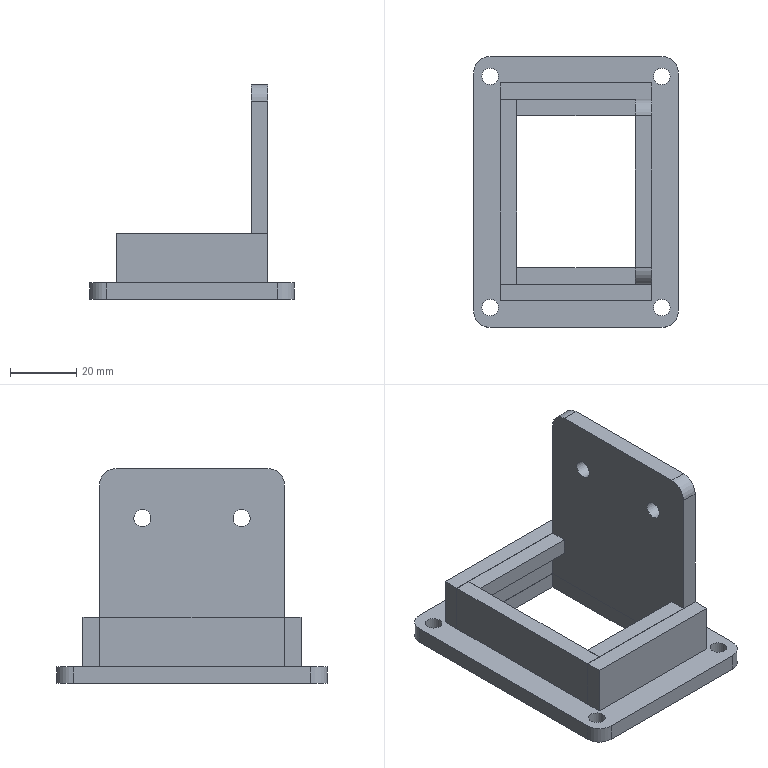Part | NX | features BREP 7 | 7 solids | 58 faces | box 62 x 82 x 65 mm | volume 44274 mm3 | plane 46 | cylinder 12 | commonest cylinder face diameters 10 x6 5 x4 5.2 x2
STEP:
#1=CARTESIAN_POINT('',(23.,-28.,5.));
#2=VERTEX_POINT('',#1);
#3=CARTESIAN_POINT('',(-23.,-28.,5.));
#4=VERTEX_POINT('',#3);
#5=CARTESIAN_POINT('',(-23.,-28.,5.));
#6=DIRECTION('',(-1.,0.,0.));
#7=VECTOR('',#6,1000.);
#8=LINE('',#5,#7);
#9=EDGE_CURVE('',#2,#4,#8,.T.);
#10=ORIENTED_EDGE('',*,*,#9,.T.);
#11=CARTESIAN_POINT('',(-23.,-28.,20.));
#12=VERTEX_POINT('',#11);
#13=CARTESIAN_POINT('',(-23.,-28.,20.));
#14=DIRECTION('',(0.,0.,-1.));
#15=VECTOR('',#14,1000.);
#16=LINE('',#13,#15);
#17=EDGE_CURVE('',#12,#4,#16,.T.);
#18=ORIENTED_EDGE('',*,*,#17,.F.);
#19=CARTESIAN_POINT('',(23.,-28.,20.));
#20=VERTEX_POINT('',#19);
#21=CARTESIAN_POINT('',(-23.,-28.,20.));
#22=DIRECTION('',(-1.,0.,0.));
#23=VECTOR('',#22,1000.);
#24=LINE('',#21,#23);
#25=EDGE_CURVE('',#20,#12,#24,.T.);
#26=ORIENTED_EDGE('',*,*,#25,.F.);
#27=CARTESIAN_POINT('',(23.,-28.,20.));
#28=DIRECTION('',(0.,0.,-1.));
#29=VECTOR('',#28,1000.);
#30=LINE('',#27,#29);
#31=EDGE_CURVE('',#20,#2,#30,.T.);
#32=ORIENTED_EDGE('',*,*,#31,.T.);
#33=EDGE_LOOP('',(#10,#18,#26,#32));
#34=FACE_BOUND('',#33,.T.);
#35=CARTESIAN_POINT('',(-23.,-28.,20.));
#36=DIRECTION('',(0.,-1.,0.));
#37=DIRECTION('',(0.,0.,-1.));
#38=AXIS2_PLACEMENT_3D('',#35,#36,#37);
#39=PLANE('',#38);
#40=ADVANCED_FACE('',(#34),#39,.F.);
#41=CARTESIAN_POINT('',(-23.,-33.,5.));
#42=VERTEX_POINT('',#41);
#43=CARTESIAN_POINT('',(-23.,-28.,5.));
#44=DIRECTION('',(0.,-1.,0.));
#45=VECTOR('',#44,1000.);
#46=LINE('',#43,#45);
#47=EDGE_CURVE('',#4,#42,#46,.T.);
#48=ORIENTED_EDGE('',*,*,#47,.T.);
#49=CARTESIAN_POINT('',(-23.,-33.,20.));
#50=VERTEX_POINT('',#49);
#51=CARTESIAN_POINT('',(-23.,-33.,20.));
#52=DIRECTION('',(0.,0.,-1.));
#53=VECTOR('',#52,1000.);
#54=LINE('',#51,#53);
#55=EDGE_CURVE('',#50,#42,#54,.T.);
#56=ORIENTED_EDGE('',*,*,#55,.F.);
#57=CARTESIAN_POINT('',(-23.,-28.,20.));
#58=DIRECTION('',(0.,-1.,0.));
#59=VECTOR('',#58,1000.);
#60=LINE('',#57,#59);
#61=EDGE_CURVE('',#12,#50,#60,.T.);
#62=ORIENTED_EDGE('',*,*,#61,.F.);
#63=ORIENTED_EDGE('',*,*,#17,.T.);
#64=EDGE_LOOP('',(#48,#56,#62,#63));
#65=FACE_BOUND('',#64,.T.);
#66=CARTESIAN_POINT('',(-23.,-28.,20.));
#67=DIRECTION('',(1.,0.,0.));
#68=DIRECTION('',(0.,0.,-1.));
#69=AXIS2_PLACEMENT_3D('',#66,#67,#68);
#70=PLANE('',#69);
#71=ADVANCED_FACE('',(#65),#70,.F.);
#72=CARTESIAN_POINT('',(23.,-33.,5.));
#73=VERTEX_POINT('',#72);
#74=CARTESIAN_POINT('',(-23.,-33.,5.));
#75=DIRECTION('',(1.,0.,0.));
#76=VECTOR('',#75,1000.);
#77=LINE('',#74,#76);
#78=EDGE_CURVE('',#42,#73,#77,.T.);
#79=ORIENTED_EDGE('',*,*,#78,.T.);
#80=CARTESIAN_POINT('',(23.,-33.,20.));
#81=VERTEX_POINT('',#80);
#82=CARTESIAN_POINT('',(23.,-33.,20.));
#83=DIRECTION('',(0.,0.,-1.));
#84=VECTOR('',#83,1000.);
#85=LINE('',#82,#84);
#86=EDGE_CURVE('',#81,#73,#85,.T.);
#87=ORIENTED_EDGE('',*,*,#86,.F.);
#88=CARTESIAN_POINT('',(-23.,-33.,20.));
#89=DIRECTION('',(1.,0.,0.));
#90=VECTOR('',#89,1000.);
#91=LINE('',#88,#90);
#92=EDGE_CURVE('',#50,#81,#91,.T.);
#93=ORIENTED_EDGE('',*,*,#92,.F.);
#94=ORIENTED_EDGE('',*,*,#55,.T.);
#95=EDGE_LOOP('',(#79,#87,#93,#94));
#96=FACE_BOUND('',#95,.T.);
#97=CARTESIAN_POINT('',(-23.,-33.,20.));
#98=DIRECTION('',(0.,1.,0.));
#99=DIRECTION('',(0.,0.,1.));
#100=AXIS2_PLACEMENT_3D('',#97,#98,#99);
#101=PLANE('',#100);
#102=ADVANCED_FACE('',(#96),#101,.F.);
#103=CARTESIAN_POINT('',(23.,-28.,5.));
#104=DIRECTION('',(0.,1.,0.));
#105=VECTOR('',#104,1000.);
#106=LINE('',#103,#105);
#107=EDGE_CURVE('',#73,#2,#106,.T.);
#108=ORIENTED_EDGE('',*,*,#107,.T.);
#109=ORIENTED_EDGE('',*,*,#31,.F.);
#110=CARTESIAN_POINT('',(23.,-28.,20.));
#111=DIRECTION('',(0.,1.,0.));
#112=VECTOR('',#111,1000.);
#113=LINE('',#110,#112);
#114=EDGE_CURVE('',#81,#20,#113,.T.);
#115=ORIENTED_EDGE('',*,*,#114,.F.);
#116=ORIENTED_EDGE('',*,*,#86,.T.);
#117=EDGE_LOOP('',(#108,#109,#115,#116));
#118=FACE_BOUND('',#117,.T.);
#119=CARTESIAN_POINT('',(23.,-28.,20.));
#120=DIRECTION('',(-1.,0.,0.));
#121=DIRECTION('',(0.,0.,1.));
#122=AXIS2_PLACEMENT_3D('',#119,#120,#121);
#123=PLANE('',#122);
#124=ADVANCED_FACE('',(#118),#123,.F.);
#125=ORIENTED_EDGE('',*,*,#25,.T.);
#126=ORIENTED_EDGE('',*,*,#61,.T.);
#127=ORIENTED_EDGE('',*,*,#92,.T.);
#128=ORIENTED_EDGE('',*,*,#114,.T.);
#129=EDGE_LOOP('',(#125,#126,#127,#128));
#130=FACE_BOUND('',#129,.T.);
#131=CARTESIAN_POINT('',(0.,0.,20.));
#132=DIRECTION('',(0.,0.,-1.));
#133=DIRECTION('',(-1.,0.,0.));
#134=AXIS2_PLACEMENT_3D('',#131,#132,#133);
#135=PLANE('',#134);
#136=ADVANCED_FACE('',(#130),#135,.F.);
#137=ORIENTED_EDGE('',*,*,#9,.F.);
#138=ORIENTED_EDGE('',*,*,#107,.F.);
#139=ORIENTED_EDGE('',*,*,#78,.F.);
#140=ORIENTED_EDGE('',*,*,#47,.F.);
#141=EDGE_LOOP('',(#137,#138,#139,#140));
#142=FACE_BOUND('',#141,.T.);
#143=CARTESIAN_POINT('',(0.,0.,5.));
#144=DIRECTION('',(0.,0.,-1.));
#145=DIRECTION('',(-1.,0.,0.));
#146=AXIS2_PLACEMENT_3D('',#143,#144,#145);
#147=PLANE('',#146);
#148=ADVANCED_FACE('',(#142),#147,.T.);
#149=CLOSED_SHELL('',(#40,#71,#102,#124,#136,#148));
#150=MANIFOLD_SOLID_BREP('',#149);
#151=CARTESIAN_POINT('',(-18.,-28.,20.));
#152=VERTEX_POINT('',#151);
#153=CARTESIAN_POINT('',(18.,-28.,20.));
#154=VERTEX_POINT('',#153);
#155=CARTESIAN_POINT('',(-18.,-28.,20.));
#156=DIRECTION('',(1.,0.,0.));
#157=VECTOR('',#156,1000.);
#158=LINE('',#155,#157);
#159=EDGE_CURVE('',#152,#154,#158,.T.);
#160=ORIENTED_EDGE('',*,*,#159,.F.);
#161=CARTESIAN_POINT('',(-18.,-28.,15.));
#162=VERTEX_POINT('',#161);
#163=CARTESIAN_POINT('',(-18.,-28.,15.));
#164=DIRECTION('',(0.,0.,1.));
#165=VECTOR('',#164,1000.);
#166=LINE('',#163,#165);
#167=EDGE_CURVE('',#162,#152,#166,.T.);
#168=ORIENTED_EDGE('',*,*,#167,.F.);
#169=CARTESIAN_POINT('',(18.,-28.,15.));
#170=VERTEX_POINT('',#169);
#171=CARTESIAN_POINT('',(-18.,-28.,15.));
#172=DIRECTION('',(1.,0.,0.));
#173=VECTOR('',#172,1000.);
#174=LINE('',#171,#173);
#175=EDGE_CURVE('',#162,#170,#174,.T.);
#176=ORIENTED_EDGE('',*,*,#175,.T.);
#177=CARTESIAN_POINT('',(18.,-28.,15.));
#178=DIRECTION('',(0.,0.,1.));
#179=VECTOR('',#178,1000.);
#180=LINE('',#177,#179);
#181=EDGE_CURVE('',#170,#154,#180,.T.);
#182=ORIENTED_EDGE('',*,*,#181,.T.);
#183=EDGE_LOOP('',(#160,#168,#176,#182));
#184=FACE_BOUND('',#183,.T.);
#185=CARTESIAN_POINT('',(-18.,-28.,15.));
#186=DIRECTION('',(0.,-1.,0.));
#187=DIRECTION('',(0.,0.,-1.));
#188=AXIS2_PLACEMENT_3D('',#185,#186,#187);
#189=PLANE('',#188);
#190=ADVANCED_FACE('',(#184),#189,.T.);
#191=CARTESIAN_POINT('',(-18.,-23.,20.));
#192=VERTEX_POINT('',#191);
#193=CARTESIAN_POINT('',(-18.,-28.,20.));
#194=DIRECTION('',(0.,-1.,0.));
#195=VECTOR('',#194,1000.);
#196=LINE('',#193,#195);
#197=EDGE_CURVE('',#192,#152,#196,.T.);
#198=ORIENTED_EDGE('',*,*,#197,.F.);
#199=CARTESIAN_POINT('',(-18.,-23.,15.));
#200=VERTEX_POINT('',#199);
#201=CARTESIAN_POINT('',(-18.,-23.,15.));
#202=DIRECTION('',(0.,0.,1.));
#203=VECTOR('',#202,1000.);
#204=LINE('',#201,#203);
#205=EDGE_CURVE('',#200,#192,#204,.T.);
#206=ORIENTED_EDGE('',*,*,#205,.F.);
#207=CARTESIAN_POINT('',(-18.,-28.,15.));
#208=DIRECTION('',(0.,-1.,0.));
#209=VECTOR('',#208,1000.);
#210=LINE('',#207,#209);
#211=EDGE_CURVE('',#200,#162,#210,.T.);
#212=ORIENTED_EDGE('',*,*,#211,.T.);
#213=ORIENTED_EDGE('',*,*,#167,.T.);
#214=EDGE_LOOP('',(#198,#206,#212,#213));
#215=FACE_BOUND('',#214,.T.);
#216=CARTESIAN_POINT('',(-18.,-28.,15.));
#217=DIRECTION('',(-1.,0.,0.));
#218=DIRECTION('',(0.,0.,1.));
#219=AXIS2_PLACEMENT_3D('',#216,#217,#218);
#220=PLANE('',#219);
#221=ADVANCED_FACE('',(#215),#220,.T.);
#222=CARTESIAN_POINT('',(18.,-23.,20.));
#223=VERTEX_POINT('',#222);
#224=CARTESIAN_POINT('',(-18.,-23.,20.));
#225=DIRECTION('',(-1.,0.,0.));
#226=VECTOR('',#225,1000.);
#227=LINE('',#224,#226);
#228=EDGE_CURVE('',#223,#192,#227,.T.);
#229=ORIENTED_EDGE('',*,*,#228,.F.);
#230=CARTESIAN_POINT('',(18.,-23.,15.));
#231=VERTEX_POINT('',#230);
#232=CARTESIAN_POINT('',(18.,-23.,15.));
#233=DIRECTION('',(0.,0.,1.));
#234=VECTOR('',#233,1000.);
#235=LINE('',#232,#234);
#236=EDGE_CURVE('',#231,#223,#235,.T.);
#237=ORIENTED_EDGE('',*,*,#236,.F.);
#238=CARTESIAN_POINT('',(-18.,-23.,15.));
#239=DIRECTION('',(-1.,0.,0.));
#240=VECTOR('',#239,1000.);
#241=LINE('',#238,#240);
#242=EDGE_CURVE('',#231,#200,#241,.T.);
#243=ORIENTED_EDGE('',*,*,#242,.T.);
#244=ORIENTED_EDGE('',*,*,#205,.T.);
#245=EDGE_LOOP('',(#229,#237,#243,#244));
#246=FACE_BOUND('',#245,.T.);
#247=CARTESIAN_POINT('',(-18.,-23.,15.));
#248=DIRECTION('',(0.,1.,0.));
#249=DIRECTION('',(0.,0.,1.));
#250=AXIS2_PLACEMENT_3D('',#247,#248,#249);
#251=PLANE('',#250);
#252=ADVANCED_FACE('',(#246),#251,.T.);
#253=CARTESIAN_POINT('',(18.,-28.,20.));
#254=DIRECTION('',(0.,1.,0.));
#255=VECTOR('',#254,1000.);
#256=LINE('',#253,#255);
#257=EDGE_CURVE('',#154,#223,#256,.T.);
#258=ORIENTED_EDGE('',*,*,#257,.F.);
#259=ORIENTED_EDGE('',*,*,#181,.F.);
#260=CARTESIAN_POINT('',(18.,-28.,15.));
#261=DIRECTION('',(0.,1.,0.));
#262=VECTOR('',#261,1000.);
#263=LINE('',#260,#262);
#264=EDGE_CURVE('',#170,#231,#263,.T.);
#265=ORIENTED_EDGE('',*,*,#264,.T.);
#266=ORIENTED_EDGE('',*,*,#236,.T.);
#267=EDGE_LOOP('',(#258,#259,#265,#266));
#268=FACE_BOUND('',#267,.T.);
#269=CARTESIAN_POINT('',(18.,-28.,15.));
#270=DIRECTION('',(1.,0.,0.));
#271=DIRECTION('',(0.,1.,0.));
#272=AXIS2_PLACEMENT_3D('',#269,#270,#271);
#273=PLANE('',#272);
#274=ADVANCED_FACE('',(#268),#273,.T.);
#275=ORIENTED_EDGE('',*,*,#175,.F.);
#276=ORIENTED_EDGE('',*,*,#211,.F.);
#277=ORIENTED_EDGE('',*,*,#242,.F.);
#278=ORIENTED_EDGE('',*,*,#264,.F.);
#279=EDGE_LOOP('',(#275,#276,#277,#278));
#280=FACE_BOUND('',#279,.T.);
#281=CARTESIAN_POINT('',(0.,0.,15.));
#282=DIRECTION('',(0.,0.,1.));
#283=DIRECTION('',(1.,0.,0.));
#284=AXIS2_PLACEMENT_3D('',#281,#282,#283);
#285=PLANE('',#284);
#286=ADVANCED_FACE('',(#280),#285,.F.);
#287=ORIENTED_EDGE('',*,*,#159,.T.);
#288=ORIENTED_EDGE('',*,*,#257,.T.);
#289=ORIENTED_EDGE('',*,*,#228,.T.);
#290=ORIENTED_EDGE('',*,*,#197,.T.);
#291=EDGE_LOOP('',(#287,#288,#289,#290));
#292=FACE_BOUND('',#291,.T.);
#293=CARTESIAN_POINT('',(0.,0.,20.));
#294=DIRECTION('',(0.,0.,1.));
#295=DIRECTION('',(1.,0.,0.));
#296=AXIS2_PLACEMENT_3D('',#293,#294,#295);
#297=PLANE('',#296);
#298=ADVANCED_FACE('',(#292),#297,.T.);
#299=CLOSED_SHELL('',(#190,#221,#252,#274,#286,#298));
#300=MANIFOLD_SOLID_BREP('',#299);
#301=CARTESIAN_POINT('',(23.,15.,47.4));
#302=VERTEX_POINT('',#301);
#303=CARTESIAN_POINT('',(23.,15.,50.));
#304=DIRECTION('',(1.,0.,0.));
#305=DIRECTION('',(0.,0.,-1.));
#306=AXIS2_PLACEMENT_3D('',#303,#304,#305);
#307=CIRCLE('',#306,2.6);
#308=EDGE_CURVE('',#302,#302,#307,.T.);
#309=ORIENTED_EDGE('',*,*,#308,.T.);
#310=EDGE_LOOP('',(#309));
#311=FACE_BOUND('',#310,.T.);
#312=CARTESIAN_POINT('',(18.,15.,47.4));
#313=VERTEX_POINT('',#312);
#314=CARTESIAN_POINT('',(18.,15.,50.));
#315=DIRECTION('',(1.,0.,0.));
#316=DIRECTION('',(0.,0.,-1.));
#317=AXIS2_PLACEMENT_3D('',#314,#315,#316);
#318=CIRCLE('',#317,2.6);
#319=EDGE_CURVE('',#313,#313,#318,.T.);
#320=ORIENTED_EDGE('',*,*,#319,.F.);
#321=EDGE_LOOP('',(#320));
#322=FACE_BOUND('',#321,.T.);
#323=CARTESIAN_POINT('',(23.,15.,50.));
#324=DIRECTION('',(1.,0.,0.));
#325=DIRECTION('',(0.,0.,-1.));
#326=AXIS2_PLACEMENT_3D('',#323,#324,#325);
#327=CYLINDRICAL_SURFACE('',#326,2.6);
#328=ADVANCED_FACE('',(#311,#322),#327,.F.);
#329=CARTESIAN_POINT('',(23.,-15.,47.4));
#330=VERTEX_POINT('',#329);
#331=CARTESIAN_POINT('',(23.,-15.,50.));
#332=DIRECTION('',(1.,0.,0.));
#333=DIRECTION('',(0.,0.,-1.));
#334=AXIS2_PLACEMENT_3D('',#331,#332,#333);
#335=CIRCLE('',#334,2.6);
#336=EDGE_CURVE('',#330,#330,#335,.T.);
#337=ORIENTED_EDGE('',*,*,#336,.T.);
#338=EDGE_LOOP('',(#337));
#339=FACE_BOUND('',#338,.T.);
#340=CARTESIAN_POINT('',(18.,-15.,47.4));
#341=VERTEX_POINT('',#340);
#342=CARTESIAN_POINT('',(18.,-15.,50.));
#343=DIRECTION('',(1.,0.,0.));
#344=DIRECTION('',(0.,0.,-1.));
#345=AXIS2_PLACEMENT_3D('',#342,#343,#344);
#346=CIRCLE('',#345,2.6);
#347=EDGE_CURVE('',#341,#341,#346,.T.);
#348=ORIENTED_EDGE('',*,*,#347,.F.);
#349=EDGE_LOOP('',(#348));
#350=FACE_BOUND('',#349,.T.);
#351=CARTESIAN_POINT('',(23.,-15.,50.));
#352=DIRECTION('',(1.,0.,0.));
#353=DIRECTION('',(0.,0.,-1.));
#354=AXIS2_PLACEMENT_3D('',#351,#352,#353);
#355=CYLINDRICAL_SURFACE('',#354,2.6);
#356=ADVANCED_FACE('',(#339,#350),#355,.F.);
#357=ORIENTED_EDGE('',*,*,#308,.F.);
#358=EDGE_LOOP('',(#357));
#359=FACE_BOUND('',#358,.T.);
#360=ORIENTED_EDGE('',*,*,#336,.F.);
#361=EDGE_LOOP('',(#360));
#362=FACE_BOUND('',#361,.T.);
#363=CARTESIAN_POINT('',(23.,28.,60.));
#364=VERTEX_POINT('',#363);
#365=CARTESIAN_POINT('',(23.,28.,5.));
#366=VERTEX_POINT('',#365);
#367=CARTESIAN_POINT('',(23.,28.,65.));
#368=DIRECTION('',(0.,0.,-1.));
#369=VECTOR('',#368,1000.);
#370=LINE('',#367,#369);
#371=EDGE_CURVE('',#364,#366,#370,.T.);
#372=ORIENTED_EDGE('',*,*,#371,.F.);
#373=CARTESIAN_POINT('',(23.,23.,65.));
#374=VERTEX_POINT('',#373);
#375=CARTESIAN_POINT('',(23.,23.,60.));
#376=DIRECTION('',(1.,0.,0.));
#377=DIRECTION('',(0.,0.,1.));
#378=AXIS2_PLACEMENT_3D('',#375,#376,#377);
#379=CIRCLE('',#378,5.);
#380=EDGE_CURVE('',#364,#374,#379,.T.);
#381=ORIENTED_EDGE('',*,*,#380,.T.);
#382=CARTESIAN_POINT('',(23.,-23.,65.));
#383=VERTEX_POINT('',#382);
#384=CARTESIAN_POINT('',(23.,-28.,65.));
#385=DIRECTION('',(0.,1.,0.));
#386=VECTOR('',#385,1000.);
#387=LINE('',#384,#386);
#388=EDGE_CURVE('',#383,#374,#387,.T.);
#389=ORIENTED_EDGE('',*,*,#388,.F.);
#390=CARTESIAN_POINT('',(23.,-28.,60.));
#391=VERTEX_POINT('',#390);
#392=CARTESIAN_POINT('',(23.,-23.,60.));
#393=DIRECTION('',(1.,0.,0.));
#394=DIRECTION('',(0.,0.,1.));
#395=AXIS2_PLACEMENT_3D('',#392,#393,#394);
#396=CIRCLE('',#395,5.);
#397=EDGE_CURVE('',#383,#391,#396,.T.);
#398=ORIENTED_EDGE('',*,*,#397,.T.);
#399=CARTESIAN_POINT('',(23.,-28.,5.));
#400=VERTEX_POINT('',#399);
#401=CARTESIAN_POINT('',(23.,-28.,65.));
#402=DIRECTION('',(0.,0.,-1.));
#403=VECTOR('',#402,1000.);
#404=LINE('',#401,#403);
#405=EDGE_CURVE('',#391,#400,#404,.T.);
#406=ORIENTED_EDGE('',*,*,#405,.T.);
#407=CARTESIAN_POINT('',(23.,28.,5.));
#408=DIRECTION('',(0.,1.,0.));
#409=VECTOR('',#408,1000.);
#410=LINE('',#407,#409);
#411=EDGE_CURVE('',#400,#366,#410,.T.);
#412=ORIENTED_EDGE('',*,*,#411,.T.);
#413=EDGE_LOOP('',(#372,#381,#389,#398,#406,#412));
#414=FACE_BOUND('',#413,.T.);
#415=CARTESIAN_POINT('',(23.,-28.,65.));
#416=DIRECTION('',(-1.,0.,0.));
#417=DIRECTION('',(0.,0.,1.));
#418=AXIS2_PLACEMENT_3D('',#415,#416,#417);
#419=PLANE('',#418);
#420=ADVANCED_FACE('',(#359,#362,#414),#419,.F.);
#421=CARTESIAN_POINT('',(18.,28.,60.));
#422=VERTEX_POINT('',#421);
#423=CARTESIAN_POINT('',(18.,28.,5.));
#424=VERTEX_POINT('',#423);
#425=CARTESIAN_POINT('',(18.,28.,65.));
#426=DIRECTION('',(0.,0.,-1.));
#427=VECTOR('',#426,1000.);
#428=LINE('',#425,#427);
#429=EDGE_CURVE('',#422,#424,#428,.T.);
#430=ORIENTED_EDGE('',*,*,#429,.F.);
#431=CARTESIAN_POINT('',(23.,28.,60.));
#432=DIRECTION('',(1.,0.,0.));
#433=VECTOR('',#432,1000.);
#434=LINE('',#431,#433);
#435=EDGE_CURVE('',#422,#364,#434,.T.);
#436=ORIENTED_EDGE('',*,*,#435,.T.);
#437=ORIENTED_EDGE('',*,*,#371,.T.);
#438=CARTESIAN_POINT('',(18.,28.,5.));
#439=DIRECTION('',(-1.,0.,0.));
#440=VECTOR('',#439,1000.);
#441=LINE('',#438,#440);
#442=EDGE_CURVE('',#366,#424,#441,.T.);
#443=ORIENTED_EDGE('',*,*,#442,.T.);
#444=EDGE_LOOP('',(#430,#436,#437,#443));
#445=FACE_BOUND('',#444,.T.);
#446=CARTESIAN_POINT('',(23.,28.,65.));
#447=DIRECTION('',(0.,-1.,0.));
#448=DIRECTION('',(0.,0.,-1.));
#449=AXIS2_PLACEMENT_3D('',#446,#447,#448);
#450=PLANE('',#449);
#451=ADVANCED_FACE('',(#445),#450,.F.);
#452=ORIENTED_EDGE('',*,*,#319,.T.);
#453=EDGE_LOOP('',(#452));
#454=FACE_BOUND('',#453,.T.);
#455=ORIENTED_EDGE('',*,*,#347,.T.);
#456=EDGE_LOOP('',(#455));
#457=FACE_BOUND('',#456,.T.);
#458=CARTESIAN_POINT('',(18.,23.,65.));
#459=VERTEX_POINT('',#458);
#460=CARTESIAN_POINT('',(18.,-23.,65.));
#461=VERTEX_POINT('',#460);
#462=CARTESIAN_POINT('',(18.,-28.,65.));
#463=DIRECTION('',(0.,-1.,0.));
#464=VECTOR('',#463,1000.);
#465=LINE('',#462,#464);
#466=EDGE_CURVE('',#459,#461,#465,.T.);
#467=ORIENTED_EDGE('',*,*,#466,.F.);
#468=CARTESIAN_POINT('',(18.,23.,60.));
#469=DIRECTION('',(-1.,0.,0.));
#470=DIRECTION('',(0.,0.,-1.));
#471=AXIS2_PLACEMENT_3D('',#468,#469,#470);
#472=CIRCLE('',#471,5.);
#473=EDGE_CURVE('',#459,#422,#472,.T.);
#474=ORIENTED_EDGE('',*,*,#473,.T.);
#475=ORIENTED_EDGE('',*,*,#429,.T.);
#476=CARTESIAN_POINT('',(18.,-28.,5.));
#477=VERTEX_POINT('',#476);
#478=CARTESIAN_POINT('',(18.,28.,5.));
#479=DIRECTION('',(0.,-1.,0.));
#480=VECTOR('',#479,1000.);
#481=LINE('',#478,#480);
#482=EDGE_CURVE('',#424,#477,#481,.T.);
#483=ORIENTED_EDGE('',*,*,#482,.T.);
#484=CARTESIAN_POINT('',(18.,-28.,60.));
#485=VERTEX_POINT('',#484);
#486=CARTESIAN_POINT('',(18.,-28.,65.));
#487=DIRECTION('',(0.,0.,-1.));
#488=VECTOR('',#487,1000.);
#489=LINE('',#486,#488);
#490=EDGE_CURVE('',#485,#477,#489,.T.);
#491=ORIENTED_EDGE('',*,*,#490,.F.);
#492=CARTESIAN_POINT('',(18.,-23.,60.));
#493=DIRECTION('',(-1.,0.,0.));
#494=DIRECTION('',(0.,0.,-1.));
#495=AXIS2_PLACEMENT_3D('',#492,#493,#494);
#496=CIRCLE('',#495,5.);
#497=EDGE_CURVE('',#485,#461,#496,.T.);
#498=ORIENTED_EDGE('',*,*,#497,.T.);
#499=EDGE_LOOP('',(#467,#474,#475,#483,#491,#498));
#500=FACE_BOUND('',#499,.T.);
#501=CARTESIAN_POINT('',(18.,-28.,65.));
#502=DIRECTION('',(1.,0.,0.));
#503=DIRECTION('',(0.,0.,-1.));
#504=AXIS2_PLACEMENT_3D('',#501,#502,#503);
#505=PLANE('',#504);
#506=ADVANCED_FACE('',(#454,#457,#500),#505,.F.);
#507=ORIENTED_EDGE('',*,*,#405,.F.);
#508=CARTESIAN_POINT('',(18.,-28.,60.));
#509=DIRECTION('',(-1.,0.,0.));
#510=VECTOR('',#509,1000.);
#511=LINE('',#508,#510);
#512=EDGE_CURVE('',#391,#485,#511,.T.);
#513=ORIENTED_EDGE('',*,*,#512,.T.);
#514=ORIENTED_EDGE('',*,*,#490,.T.);
#515=CARTESIAN_POINT('',(18.,-28.,5.));
#516=DIRECTION('',(1.,0.,0.));
#517=VECTOR('',#516,1000.);
#518=LINE('',#515,#517);
#519=EDGE_CURVE('',#477,#400,#518,.T.);
#520=ORIENTED_EDGE('',*,*,#519,.T.);
#521=EDGE_LOOP('',(#507,#513,#514,#520));
#522=FACE_BOUND('',#521,.T.);
#523=CARTESIAN_POINT('',(23.,-28.,65.));
#524=DIRECTION('',(0.,1.,0.));
#525=DIRECTION('',(0.,0.,1.));
#526=AXIS2_PLACEMENT_3D('',#523,#524,#525);
#527=PLANE('',#526);
#528=ADVANCED_FACE('',(#522),#527,.F.);
#529=ORIENTED_EDGE('',*,*,#388,.T.);
#530=CARTESIAN_POINT('',(18.,23.,65.));
#531=DIRECTION('',(-1.,0.,0.));
#532=VECTOR('',#531,1000.);
#533=LINE('',#530,#532);
#534=EDGE_CURVE('',#374,#459,#533,.T.);
#535=ORIENTED_EDGE('',*,*,#534,.T.);
#536=ORIENTED_EDGE('',*,*,#466,.T.);
#537=CARTESIAN_POINT('',(23.,-23.,65.));
#538=DIRECTION('',(1.,0.,0.));
#539=VECTOR('',#538,1000.);
#540=LINE('',#537,#539);
#541=EDGE_CURVE('',#461,#383,#540,.T.);
#542=ORIENTED_EDGE('',*,*,#541,.T.);
#543=EDGE_LOOP('',(#529,#535,#536,#542));
#544=FACE_BOUND('',#543,.T.);
#545=CARTESIAN_POINT('',(0.,0.,65.));
#546=DIRECTION('',(0.,0.,1.));
#547=DIRECTION('',(1.,0.,0.));
#548=AXIS2_PLACEMENT_3D('',#545,#546,#547);
#549=PLANE('',#548);
#550=ADVANCED_FACE('',(#544),#549,.T.);
#551=ORIENTED_EDGE('',*,*,#380,.F.);
#552=ORIENTED_EDGE('',*,*,#435,.F.);
#553=ORIENTED_EDGE('',*,*,#473,.F.);
#554=ORIENTED_EDGE('',*,*,#534,.F.);
#555=EDGE_LOOP('',(#551,#552,#553,#554));
#556=FACE_BOUND('',#555,.T.);
#557=CARTESIAN_POINT('',(0.,23.,60.));
#558=DIRECTION('',(1.,0.,0.));
#559=DIRECTION('',(0.,0.,-1.));
#560=AXIS2_PLACEMENT_3D('',#557,#558,#559);
#561=CYLINDRICAL_SURFACE('',#560,5.);
#562=ADVANCED_FACE('',(#556),#561,.T.);
#563=ORIENTED_EDGE('',*,*,#497,.F.);
#564=ORIENTED_EDGE('',*,*,#512,.F.);
#565=ORIENTED_EDGE('',*,*,#397,.F.);
#566=ORIENTED_EDGE('',*,*,#541,.F.);
#567=EDGE_LOOP('',(#563,#564,#565,#566));
#568=FACE_BOUND('',#567,.T.);
#569=CARTESIAN_POINT('',(0.,-23.,60.));
#570=DIRECTION('',(-1.,0.,0.));
#571=DIRECTION('',(0.,0.,1.));
#572=AXIS2_PLACEMENT_3D('',#569,#570,#571);
#573=CYLINDRICAL_SURFACE('',#572,5.);
#574=ADVANCED_FACE('',(#568),#573,.T.);
#575=ORIENTED_EDGE('',*,*,#442,.F.);
#576=ORIENTED_EDGE('',*,*,#411,.F.);
#577=ORIENTED_EDGE('',*,*,#519,.F.);
#578=ORIENTED_EDGE('',*,*,#482,.F.);
#579=EDGE_LOOP('',(#575,#576,#577,#578));
#580=FACE_BOUND('',#579,.T.);
#581=CARTESIAN_POINT('',(0.,0.,5.));
#582=DIRECTION('',(0.,0.,-1.));
#583=DIRECTION('',(-1.,0.,0.));
#584=AXIS2_PLACEMENT_3D('',#581,#582,#583);
#585=PLANE('',#584);
#586=ADVANCED_FACE('',(#580),#585,.T.);
#587=CLOSED_SHELL('',(#328,#356,#420,#451,#506,#528,#550,#562,#574,#586));
#588=MANIFOLD_SOLID_BREP('',#587);
#589=CARTESIAN_POINT('',(-18.,-28.,5.));
#590=VERTEX_POINT('',#589);
#591=CARTESIAN_POINT('',(-18.,28.,5.));
#592=VERTEX_POINT('',#591);
#593=CARTESIAN_POINT('',(-18.,28.,5.));
#594=DIRECTION('',(0.,1.,0.));
#595=VECTOR('',#594,1000.);
#596=LINE('',#593,#595);
#597=EDGE_CURVE('',#590,#592,#596,.T.);
#598=ORIENTED_EDGE('',*,*,#597,.T.);
#599=CARTESIAN_POINT('',(-18.,28.,20.));
#600=VERTEX_POINT('',#599);
#601=CARTESIAN_POINT('',(-18.,28.,20.));
#602=DIRECTION('',(0.,0.,-1.));
#603=VECTOR('',#602,1000.);
#604=LINE('',#601,#603);
#605=EDGE_CURVE('',#600,#592,#604,.T.);
#606=ORIENTED_EDGE('',*,*,#605,.F.);
#607=CARTESIAN_POINT('',(-18.,-28.,20.));
#608=VERTEX_POINT('',#607);
#609=CARTESIAN_POINT('',(-18.,28.,20.));
#610=DIRECTION('',(0.,1.,0.));
#611=VECTOR('',#610,1000.);
#612=LINE('',#609,#611);
#613=EDGE_CURVE('',#608,#600,#612,.T.);
#614=ORIENTED_EDGE('',*,*,#613,.F.);
#615=CARTESIAN_POINT('',(-18.,-28.,20.));
#616=DIRECTION('',(0.,0.,-1.));
#617=VECTOR('',#616,1000.);
#618=LINE('',#615,#617);
#619=EDGE_CURVE('',#608,#590,#618,.T.);
#620=ORIENTED_EDGE('',*,*,#619,.T.);
#621=EDGE_LOOP('',(#598,#606,#614,#620));
#622=FACE_BOUND('',#621,.T.);
#623=CARTESIAN_POINT('',(-18.,28.,20.));
#624=DIRECTION('',(-1.,0.,0.));
#625=DIRECTION('',(0.,0.,1.));
#626=AXIS2_PLACEMENT_3D('',#623,#624,#625);
#627=PLANE('',#626);
#628=ADVANCED_FACE('',(#622),#627,.F.);
#629=CARTESIAN_POINT('',(-23.,28.,5.));
#630=VERTEX_POINT('',#629);
#631=CARTESIAN_POINT('',(-18.,28.,5.));
#632=DIRECTION('',(-1.,0.,0.));
#633=VECTOR('',#632,1000.);
#634=LINE('',#631,#633);
#635=EDGE_CURVE('',#592,#630,#634,.T.);
#636=ORIENTED_EDGE('',*,*,#635,.T.);
#637=CARTESIAN_POINT('',(-23.,28.,20.));
#638=VERTEX_POINT('',#637);
#639=CARTESIAN_POINT('',(-23.,28.,20.));
#640=DIRECTION('',(0.,0.,-1.));
#641=VECTOR('',#640,1000.);
#642=LINE('',#639,#641);
#643=EDGE_CURVE('',#638,#630,#642,.T.);
#644=ORIENTED_EDGE('',*,*,#643,.F.);
#645=CARTESIAN_POINT('',(-18.,28.,20.));
#646=DIRECTION('',(-1.,0.,0.));
#647=VECTOR('',#646,1000.);
#648=LINE('',#645,#647);
#649=EDGE_CURVE('',#600,#638,#648,.T.);
#650=ORIENTED_EDGE('',*,*,#649,.F.);
#651=ORIENTED_EDGE('',*,*,#605,.T.);
#652=EDGE_LOOP('',(#636,#644,#650,#651));
#653=FACE_BOUND('',#652,.T.);
#654=CARTESIAN_POINT('',(-18.,28.,20.));
#655=DIRECTION('',(0.,-1.,0.));
#656=DIRECTION('',(0.,0.,-1.));
#657=AXIS2_PLACEMENT_3D('',#654,#655,#656);
#658=PLANE('',#657);
#659=ADVANCED_FACE('',(#653),#658,.F.);
#660=CARTESIAN_POINT('',(-23.,-28.,5.));
#661=VERTEX_POINT('',#660);
#662=CARTESIAN_POINT('',(-23.,28.,5.));
#663=DIRECTION('',(0.,-1.,0.));
#664=VECTOR('',#663,1000.);
#665=LINE('',#662,#664);
#666=EDGE_CURVE('',#630,#661,#665,.T.);
#667=ORIENTED_EDGE('',*,*,#666,.T.);
#668=CARTESIAN_POINT('',(-23.,-28.,20.));
#669=VERTEX_POINT('',#668);
#670=CARTESIAN_POINT('',(-23.,-28.,20.));
#671=DIRECTION('',(0.,0.,-1.));
#672=VECTOR('',#671,1000.);
#673=LINE('',#670,#672);
#674=EDGE_CURVE('',#669,#661,#673,.T.);
#675=ORIENTED_EDGE('',*,*,#674,.F.);
#676=CARTESIAN_POINT('',(-23.,28.,20.));
#677=DIRECTION('',(0.,-1.,0.));
#678=VECTOR('',#677,1000.);
#679=LINE('',#676,#678);
#680=EDGE_CURVE('',#638,#669,#679,.T.);
#681=ORIENTED_EDGE('',*,*,#680,.F.);
#682=ORIENTED_EDGE('',*,*,#643,.T.);
#683=EDGE_LOOP('',(#667,#675,#681,#682));
#684=FACE_BOUND('',#683,.T.);
#685=CARTESIAN_POINT('',(-23.,28.,20.));
#686=DIRECTION('',(1.,0.,0.));
#687=DIRECTION('',(0.,1.,0.));
#688=AXIS2_PLACEMENT_3D('',#685,#686,#687);
#689=PLANE('',#688);
#690=ADVANCED_FACE('',(#684),#689,.F.);
#691=CARTESIAN_POINT('',(-18.,-28.,5.));
#692=DIRECTION('',(1.,0.,0.));
#693=VECTOR('',#692,1000.);
#694=LINE('',#691,#693);
#695=EDGE_CURVE('',#661,#590,#694,.T.);
#696=ORIENTED_EDGE('',*,*,#695,.T.);
#697=ORIENTED_EDGE('',*,*,#619,.F.);
#698=CARTESIAN_POINT('',(-18.,-28.,20.));
#699=DIRECTION('',(1.,0.,0.));
#700=VECTOR('',#699,1000.);
#701=LINE('',#698,#700);
#702=EDGE_CURVE('',#669,#608,#701,.T.);
#703=ORIENTED_EDGE('',*,*,#702,.F.);
#704=ORIENTED_EDGE('',*,*,#674,.T.);
#705=EDGE_LOOP('',(#696,#697,#703,#704));
#706=FACE_BOUND('',#705,.T.);
#707=CARTESIAN_POINT('',(-18.,-28.,20.));
#708=DIRECTION('',(0.,1.,0.));
#709=DIRECTION('',(0.,0.,1.));
#710=AXIS2_PLACEMENT_3D('',#707,#708,#709);
#711=PLANE('',#710);
#712=ADVANCED_FACE('',(#706),#711,.F.);
#713=ORIENTED_EDGE('',*,*,#613,.T.);
#714=ORIENTED_EDGE('',*,*,#649,.T.);
#715=ORIENTED_EDGE('',*,*,#680,.T.);
#716=ORIENTED_EDGE('',*,*,#702,.T.);
#717=EDGE_LOOP('',(#713,#714,#715,#716));
#718=FACE_BOUND('',#717,.T.);
#719=CARTESIAN_POINT('',(0.,0.,20.));
#720=DIRECTION('',(0.,0.,-1.));
#721=DIRECTION('',(-1.,0.,0.));
#722=AXIS2_PLACEMENT_3D('',#719,#720,#721);
#723=PLANE('',#722);
#724=ADVANCED_FACE('',(#718),#723,.F.);
#725=ORIENTED_EDGE('',*,*,#597,.F.);
#726=ORIENTED_EDGE('',*,*,#695,.F.);
#727=ORIENTED_EDGE('',*,*,#666,.F.);
#728=ORIENTED_EDGE('',*,*,#635,.F.);
#729=EDGE_LOOP('',(#725,#726,#727,#728));
#730=FACE_BOUND('',#729,.T.);
#731=CARTESIAN_POINT('',(0.,0.,5.));
#732=DIRECTION('',(0.,0.,-1.));
#733=DIRECTION('',(-1.,0.,0.));
#734=AXIS2_PLACEMENT_3D('',#731,#732,#733);
#735=PLANE('',#734);
#736=ADVANCED_FACE('',(#730),#735,.T.);
#737=CLOSED_SHELL('',(#628,#659,#690,#712,#724,#736));
#738=MANIFOLD_SOLID_BREP('',#737);
#739=CARTESIAN_POINT('',(23.5,35.,0.));
#740=VERTEX_POINT('',#739);
#741=CARTESIAN_POINT('',(26.,35.,0.));
#742=DIRECTION('',(0.,0.,-1.));
#743=DIRECTION('',(-1.,0.,0.));
#744=AXIS2_PLACEMENT_3D('',#741,#742,#743);
#745=CIRCLE('',#744,2.5);
#746=EDGE_CURVE('',#740,#740,#745,.T.);
#747=ORIENTED_EDGE('',*,*,#746,.T.);
#748=EDGE_LOOP('',(#747));
#749=FACE_BOUND('',#748,.T.);
#750=CARTESIAN_POINT('',(28.5,35.,5.));
#751=VERTEX_POINT('',#750);
#752=CARTESIAN_POINT('',(26.,35.,5.));
#753=DIRECTION('',(0.,0.,-1.));
#754=DIRECTION('',(1.,0.,0.));
#755=AXIS2_PLACEMENT_3D('',#752,#753,#754);
#756=CIRCLE('',#755,2.5);
#757=EDGE_CURVE('',#751,#751,#756,.T.);
#758=ORIENTED_EDGE('',*,*,#757,.F.);
#759=EDGE_LOOP('',(#758));
#760=FACE_BOUND('',#759,.T.);
#761=CARTESIAN_POINT('',(26.,35.,0.));
#762=DIRECTION('',(0.,0.,-1.));
#763=DIRECTION('',(-1.,0.,0.));
#764=AXIS2_PLACEMENT_3D('',#761,#762,#763);
#765=CYLINDRICAL_SURFACE('',#764,2.5);
#766=ADVANCED_FACE('',(#749,#760),#765,.F.);
#767=CARTESIAN_POINT('',(-28.5,35.,0.));
#768=VERTEX_POINT('',#767);
#769=CARTESIAN_POINT('',(-26.,35.,0.));
#770=DIRECTION('',(0.,0.,-1.));
#771=DIRECTION('',(-1.,0.,0.));
#772=AXIS2_PLACEMENT_3D('',#769,#770,#771);
#773=CIRCLE('',#772,2.5);
#774=EDGE_CURVE('',#768,#768,#773,.T.);
#775=ORIENTED_EDGE('',*,*,#774,.T.);
#776=EDGE_LOOP('',(#775));
#777=FACE_BOUND('',#776,.T.);
#778=CARTESIAN_POINT('',(-23.5,35.,5.));
#779=VERTEX_POINT('',#778);
#780=CARTESIAN_POINT('',(-26.,35.,5.));
#781=DIRECTION('',(0.,0.,-1.));
#782=DIRECTION('',(1.,0.,0.));
#783=AXIS2_PLACEMENT_3D('',#780,#781,#782);
#784=CIRCLE('',#783,2.5);
#785=EDGE_CURVE('',#779,#779,#784,.T.);
#786=ORIENTED_EDGE('',*,*,#785,.F.);
#787=EDGE_LOOP('',(#786));
#788=FACE_BOUND('',#787,.T.);
#789=CARTESIAN_POINT('',(-26.,35.,0.));
#790=DIRECTION('',(0.,0.,-1.));
#791=DIRECTION('',(-1.,0.,0.));
#792=AXIS2_PLACEMENT_3D('',#789,#790,#791);
#793=CYLINDRICAL_SURFACE('',#792,2.5);
#794=ADVANCED_FACE('',(#777,#788),#793,.F.);
#795=CARTESIAN_POINT('',(-28.5,-35.,0.));
#796=VERTEX_POINT('',#795);
#797=CARTESIAN_POINT('',(-26.,-35.,0.));
#798=DIRECTION('',(0.,0.,-1.));
#799=DIRECTION('',(-1.,0.,0.));
#800=AXIS2_PLACEMENT_3D('',#797,#798,#799);
#801=CIRCLE('',#800,2.5);
#802=EDGE_CURVE('',#796,#796,#801,.T.);
#803=ORIENTED_EDGE('',*,*,#802,.T.);
#804=EDGE_LOOP('',(#803));
#805=FACE_BOUND('',#804,.T.);
#806=CARTESIAN_POINT('',(-23.5,-35.,5.));
#807=VERTEX_POINT('',#806);
#808=CARTESIAN_POINT('',(-26.,-35.,5.));
#809=DIRECTION('',(0.,0.,-1.));
#810=DIRECTION('',(1.,0.,0.));
#811=AXIS2_PLACEMENT_3D('',#808,#809,#810);
#812=CIRCLE('',#811,2.5);
#813=EDGE_CURVE('',#807,#807,#812,.T.);
#814=ORIENTED_EDGE('',*,*,#813,.F.);
#815=EDGE_LOOP('',(#814));
#816=FACE_BOUND('',#815,.T.);
#817=CARTESIAN_POINT('',(-26.,-35.,0.));
#818=DIRECTION('',(0.,0.,-1.));
#819=DIRECTION('',(-1.,0.,0.));
#820=AXIS2_PLACEMENT_3D('',#817,#818,#819);
#821=CYLINDRICAL_SURFACE('',#820,2.5);
#822=ADVANCED_FACE('',(#805,#816),#821,.F.);
#823=CARTESIAN_POINT('',(23.5,-35.,0.));
#824=VERTEX_POINT('',#823);
#825=CARTESIAN_POINT('',(26.,-35.,0.));
#826=DIRECTION('',(0.,0.,-1.));
#827=DIRECTION('',(-1.,0.,0.));
#828=AXIS2_PLACEMENT_3D('',#825,#826,#827);
#829=CIRCLE('',#828,2.5);
#830=EDGE_CURVE('',#824,#824,#829,.T.);
#831=ORIENTED_EDGE('',*,*,#830,.T.);
#832=EDGE_LOOP('',(#831));
#833=FACE_BOUND('',#832,.T.);
#834=CARTESIAN_POINT('',(28.5,-35.,5.));
#835=VERTEX_POINT('',#834);
#836=CARTESIAN_POINT('',(26.,-35.,5.));
#837=DIRECTION('',(0.,0.,-1.));
#838=DIRECTION('',(1.,0.,0.));
#839=AXIS2_PLACEMENT_3D('',#836,#837,#838);
#840=CIRCLE('',#839,2.5);
#841=EDGE_CURVE('',#835,#835,#840,.T.);
#842=ORIENTED_EDGE('',*,*,#841,.F.);
#843=EDGE_LOOP('',(#842));
#844=FACE_BOUND('',#843,.T.);
#845=CARTESIAN_POINT('',(26.,-35.,0.));
#846=DIRECTION('',(0.,0.,-1.));
#847=DIRECTION('',(-1.,0.,0.));
#848=AXIS2_PLACEMENT_3D('',#845,#846,#847);
#849=CYLINDRICAL_SURFACE('',#848,2.5);
#850=ADVANCED_FACE('',(#833,#844),#849,.F.);
#851=ORIENTED_EDGE('',*,*,#813,.T.);
#852=EDGE_LOOP('',(#851));
#853=FACE_BOUND('',#852,.T.);
#854=ORIENTED_EDGE('',*,*,#841,.T.);
#855=EDGE_LOOP('',(#854));
#856=FACE_BOUND('',#855,.T.);
#857=CARTESIAN_POINT('',(-31.,36.,5.));
#858=VERTEX_POINT('',#857);
#859=CARTESIAN_POINT('',(-31.,-36.,5.));
#860=VERTEX_POINT('',#859);
#861=CARTESIAN_POINT('',(-31.,-41.,5.));
#862=DIRECTION('',(0.,-1.,0.));
#863=VECTOR('',#862,1000.);
#864=LINE('',#861,#863);
#865=EDGE_CURVE('',#858,#860,#864,.T.);
#866=ORIENTED_EDGE('',*,*,#865,.T.);
#867=CARTESIAN_POINT('',(-26.,-41.,5.));
#868=VERTEX_POINT('',#867);
#869=CARTESIAN_POINT('',(-26.,-36.,5.));
#870=DIRECTION('',(0.,0.,1.));
#871=DIRECTION('',(1.,0.,0.));
#872=AXIS2_PLACEMENT_3D('',#869,#870,#871);
#873=CIRCLE('',#872,5.);
#874=EDGE_CURVE('',#860,#868,#873,.T.);
#875=ORIENTED_EDGE('',*,*,#874,.T.);
#876=CARTESIAN_POINT('',(26.,-41.,5.));
#877=VERTEX_POINT('',#876);
#878=CARTESIAN_POINT('',(-31.,-41.,5.));
#879=DIRECTION('',(1.,0.,0.));
#880=VECTOR('',#879,1000.);
#881=LINE('',#878,#880);
#882=EDGE_CURVE('',#868,#877,#881,.T.);
#883=ORIENTED_EDGE('',*,*,#882,.T.);
#884=CARTESIAN_POINT('',(31.,-36.,5.));
#885=VERTEX_POINT('',#884);
#886=CARTESIAN_POINT('',(26.,-36.,5.));
#887=DIRECTION('',(0.,0.,1.));
#888=DIRECTION('',(1.,0.,0.));
#889=AXIS2_PLACEMENT_3D('',#886,#887,#888);
#890=CIRCLE('',#889,5.);
#891=EDGE_CURVE('',#877,#885,#890,.T.);
#892=ORIENTED_EDGE('',*,*,#891,.T.);
#893=CARTESIAN_POINT('',(31.,36.,5.));
#894=VERTEX_POINT('',#893);
#895=CARTESIAN_POINT('',(31.,-41.,5.));
#896=DIRECTION('',(0.,1.,0.));
#897=VECTOR('',#896,1000.);
#898=LINE('',#895,#897);
#899=EDGE_CURVE('',#885,#894,#898,.T.);
#900=ORIENTED_EDGE('',*,*,#899,.T.);
#901=CARTESIAN_POINT('',(26.,41.,5.));
#902=VERTEX_POINT('',#901);
#903=CARTESIAN_POINT('',(26.,36.,5.));
#904=DIRECTION('',(0.,0.,1.));
#905=DIRECTION('',(1.,0.,0.));
#906=AXIS2_PLACEMENT_3D('',#903,#904,#905);
#907=CIRCLE('',#906,5.);
#908=EDGE_CURVE('',#894,#902,#907,.T.);
#909=ORIENTED_EDGE('',*,*,#908,.T.);
#910=CARTESIAN_POINT('',(-26.,41.,5.));
#911=VERTEX_POINT('',#910);
#912=CARTESIAN_POINT('',(-31.,41.,5.));
#913=DIRECTION('',(-1.,0.,0.));
#914=VECTOR('',#913,1000.);
#915=LINE('',#912,#914);
#916=EDGE_CURVE('',#902,#911,#915,.T.);
#917=ORIENTED_EDGE('',*,*,#916,.T.);
#918=CARTESIAN_POINT('',(-26.,36.,5.));
#919=DIRECTION('',(0.,0.,1.));
#920=DIRECTION('',(1.,0.,0.));
#921=AXIS2_PLACEMENT_3D('',#918,#919,#920);
#922=CIRCLE('',#921,5.);
#923=EDGE_CURVE('',#911,#858,#922,.T.);
#924=ORIENTED_EDGE('',*,*,#923,.T.);
#925=EDGE_LOOP('',(#866,#875,#883,#892,#900,#909,#917,#924));
#926=FACE_BOUND('',#925,.T.);
#927=CARTESIAN_POINT('',(-18.,28.,5.));
#928=VERTEX_POINT('',#927);
#929=CARTESIAN_POINT('',(-18.,-28.,5.));
#930=VERTEX_POINT('',#929);
#931=CARTESIAN_POINT('',(-18.,-28.,5.));
#932=DIRECTION('',(0.,-1.,0.));
#933=VECTOR('',#932,1000.);
#934=LINE('',#931,#933);
#935=EDGE_CURVE('',#928,#930,#934,.T.);
#936=ORIENTED_EDGE('',*,*,#935,.F.);
#937=CARTESIAN_POINT('',(18.,28.,5.));
#938=VERTEX_POINT('',#937);
#939=CARTESIAN_POINT('',(-18.,28.,5.));
#940=DIRECTION('',(-1.,0.,0.));
#941=VECTOR('',#940,1000.);
#942=LINE('',#939,#941);
#943=EDGE_CURVE('',#938,#928,#942,.T.);
#944=ORIENTED_EDGE('',*,*,#943,.F.);
#945=CARTESIAN_POINT('',(18.,-28.,5.));
#946=VERTEX_POINT('',#945);
#947=CARTESIAN_POINT('',(18.,-28.,5.));
#948=DIRECTION('',(0.,1.,0.));
#949=VECTOR('',#948,1000.);
#950=LINE('',#947,#949);
#951=EDGE_CURVE('',#946,#938,#950,.T.);
#952=ORIENTED_EDGE('',*,*,#951,.F.);
#953=CARTESIAN_POINT('',(-18.,-28.,5.));
#954=DIRECTION('',(1.,0.,0.));
#955=VECTOR('',#954,1000.);
#956=LINE('',#953,#955);
#957=EDGE_CURVE('',#930,#946,#956,.T.);
#958=ORIENTED_EDGE('',*,*,#957,.F.);
#959=EDGE_LOOP('',(#936,#944,#952,#958));
#960=FACE_BOUND('',#959,.T.);
#961=ORIENTED_EDGE('',*,*,#785,.T.);
#962=EDGE_LOOP('',(#961));
#963=FACE_BOUND('',#962,.T.);
#964=ORIENTED_EDGE('',*,*,#757,.T.);
#965=EDGE_LOOP('',(#964));
#966=FACE_BOUND('',#965,.T.);
#967=CARTESIAN_POINT('',(0.,0.,5.));
#968=DIRECTION('',(0.,0.,1.));
#969=DIRECTION('',(1.,0.,0.));
#970=AXIS2_PLACEMENT_3D('',#967,#968,#969);
#971=PLANE('',#970);
#972=ADVANCED_FACE('',(#853,#856,#926,#960,#963,#966),#971,.T.);
#973=ORIENTED_EDGE('',*,*,#746,.F.);
#974=EDGE_LOOP('',(#973));
#975=FACE_BOUND('',#974,.T.);
#976=ORIENTED_EDGE('',*,*,#774,.F.);
#977=EDGE_LOOP('',(#976));
#978=FACE_BOUND('',#977,.T.);
#979=ORIENTED_EDGE('',*,*,#802,.F.);
#980=EDGE_LOOP('',(#979));
#981=FACE_BOUND('',#980,.T.);
#982=ORIENTED_EDGE('',*,*,#830,.F.);
#983=EDGE_LOOP('',(#982));
#984=FACE_BOUND('',#983,.T.);
#985=CARTESIAN_POINT('',(-26.,-41.,0.));
#986=VERTEX_POINT('',#985);
#987=CARTESIAN_POINT('',(26.,-41.,0.));
#988=VERTEX_POINT('',#987);
#989=CARTESIAN_POINT('',(-31.,-41.,0.));
#990=DIRECTION('',(1.,0.,0.));
#991=VECTOR('',#990,1000.);
#992=LINE('',#989,#991);
#993=EDGE_CURVE('',#986,#988,#992,.T.);
#994=ORIENTED_EDGE('',*,*,#993,.F.);
#995=CARTESIAN_POINT('',(-31.,-36.,0.));
#996=VERTEX_POINT('',#995);
#997=CARTESIAN_POINT('',(-26.,-36.,0.));
#998=DIRECTION('',(0.,0.,-1.));
#999=DIRECTION('',(1.,0.,0.));
#1000=AXIS2_PLACEMENT_3D('',#997,#998,#999);
#1001=CIRCLE('',#1000,5.);
#1002=EDGE_CURVE('',#986,#996,#1001,.T.);
#1003=ORIENTED_EDGE('',*,*,#1002,.T.);
#1004=CARTESIAN_POINT('',(-31.,36.,0.));
#1005=VERTEX_POINT('',#1004);
#1006=CARTESIAN_POINT('',(-31.,-41.,0.));
#1007=DIRECTION('',(0.,-1.,0.));
#1008=VECTOR('',#1007,1000.);
#1009=LINE('',#1006,#1008);
#1010=EDGE_CURVE('',#1005,#996,#1009,.T.);
#1011=ORIENTED_EDGE('',*,*,#1010,.F.);
#1012=CARTESIAN_POINT('',(-26.,41.,0.));
#1013=VERTEX_POINT('',#1012);
#1014=CARTESIAN_POINT('',(-26.,36.,0.));
#1015=DIRECTION('',(0.,0.,-1.));
#1016=DIRECTION('',(1.,0.,0.));
#1017=AXIS2_PLACEMENT_3D('',#1014,#1015,#1016);
#1018=CIRCLE('',#1017,5.);
#1019=EDGE_CURVE('',#1005,#1013,#1018,.T.);
#1020=ORIENTED_EDGE('',*,*,#1019,.T.);
#1021=CARTESIAN_POINT('',(26.,41.,0.));
#1022=VERTEX_POINT('',#1021);
#1023=CARTESIAN_POINT('',(-31.,41.,0.));
#1024=DIRECTION('',(-1.,0.,0.));
#1025=VECTOR('',#1024,1000.);
#1026=LINE('',#1023,#1025);
#1027=EDGE_CURVE('',#1022,#1013,#1026,.T.);
#1028=ORIENTED_EDGE('',*,*,#1027,.F.);
#1029=CARTESIAN_POINT('',(31.,36.,0.));
#1030=VERTEX_POINT('',#1029);
#1031=CARTESIAN_POINT('',(26.,36.,0.));
#1032=DIRECTION('',(0.,0.,-1.));
#1033=DIRECTION('',(1.,0.,0.));
#1034=AXIS2_PLACEMENT_3D('',#1031,#1032,#1033);
#1035=CIRCLE('',#1034,5.);
#1036=EDGE_CURVE('',#1022,#1030,#1035,.T.);
#1037=ORIENTED_EDGE('',*,*,#1036,.T.);
#1038=CARTESIAN_POINT('',(31.,-36.,0.));
#1039=VERTEX_POINT('',#1038);
#1040=CARTESIAN_POINT('',(31.,-41.,0.));
#1041=DIRECTION('',(0.,1.,0.));
#1042=VECTOR('',#1041,1000.);
#1043=LINE('',#1040,#1042);
#1044=EDGE_CURVE('',#1039,#1030,#1043,.T.);
#1045=ORIENTED_EDGE('',*,*,#1044,.F.);
#1046=CARTESIAN_POINT('',(26.,-36.,0.));
#1047=DIRECTION('',(0.,0.,-1.));
#1048=DIRECTION('',(1.,0.,0.));
#1049=AXIS2_PLACEMENT_3D('',#1046,#1047,#1048);
#1050=CIRCLE('',#1049,5.);
#1051=EDGE_CURVE('',#1039,#988,#1050,.T.);
#1052=ORIENTED_EDGE('',*,*,#1051,.T.);
#1053=EDGE_LOOP('',(#994,#1003,#1011,#1020,#1028,#1037,#1045,#1052));
#1054=FACE_BOUND('',#1053,.T.);
#1055=CARTESIAN_POINT('',(18.,28.,0.));
#1056=VERTEX_POINT('',#1055);
#1057=CARTESIAN_POINT('',(-18.,28.,0.));
#1058=VERTEX_POINT('',#1057);
#1059=CARTESIAN_POINT('',(-18.,28.,0.));
#1060=DIRECTION('',(-1.,0.,0.));
#1061=VECTOR('',#1060,1000.);
#1062=LINE('',#1059,#1061);
#1063=EDGE_CURVE('',#1056,#1058,#1062,.T.);
#1064=ORIENTED_EDGE('',*,*,#1063,.T.);
#1065=CARTESIAN_POINT('',(-18.,-28.,0.));
#1066=VERTEX_POINT('',#1065);
#1067=CARTESIAN_POINT('',(-18.,-28.,0.));
#1068=DIRECTION('',(0.,-1.,0.));
#1069=VECTOR('',#1068,1000.);
#1070=LINE('',#1067,#1069);
#1071=EDGE_CURVE('',#1058,#1066,#1070,.T.);
#1072=ORIENTED_EDGE('',*,*,#1071,.T.);
#1073=CARTESIAN_POINT('',(18.,-28.,0.));
#1074=VERTEX_POINT('',#1073);
#1075=CARTESIAN_POINT('',(-18.,-28.,0.));
#1076=DIRECTION('',(1.,0.,0.));
#1077=VECTOR('',#1076,1000.);
#1078=LINE('',#1075,#1077);
#1079=EDGE_CURVE('',#1066,#1074,#1078,.T.);
#1080=ORIENTED_EDGE('',*,*,#1079,.T.);
#1081=CARTESIAN_POINT('',(18.,-28.,0.));
#1082=DIRECTION('',(0.,1.,0.));
#1083=VECTOR('',#1082,1000.);
#1084=LINE('',#1081,#1083);
#1085=EDGE_CURVE('',#1074,#1056,#1084,.T.);
#1086=ORIENTED_EDGE('',*,*,#1085,.T.);
#1087=EDGE_LOOP('',(#1064,#1072,#1080,#1086));
#1088=FACE_BOUND('',#1087,.T.);
#1089=CARTESIAN_POINT('',(0.,0.,0.));
#1090=DIRECTION('',(0.,0.,1.));
#1091=DIRECTION('',(1.,0.,0.));
#1092=AXIS2_PLACEMENT_3D('',#1089,#1090,#1091);
#1093=PLANE('',#1092);
#1094=ADVANCED_FACE('',(#975,#978,#981,#984,#1054,#1088),#1093,.F.);
#1095=ORIENTED_EDGE('',*,*,#882,.F.);
#1096=CARTESIAN_POINT('',(-26.,-41.,5.));
#1097=DIRECTION('',(0.,0.,-1.));
#1098=VECTOR('',#1097,1000.);
#1099=LINE('',#1096,#1098);
#1100=EDGE_CURVE('',#868,#986,#1099,.T.);
#1101=ORIENTED_EDGE('',*,*,#1100,.T.);
#1102=ORIENTED_EDGE('',*,*,#993,.T.);
#1103=CARTESIAN_POINT('',(26.,-41.,5.));
#1104=DIRECTION('',(0.,0.,1.));
#1105=VECTOR('',#1104,1000.);
#1106=LINE('',#1103,#1105);
#1107=EDGE_CURVE('',#988,#877,#1106,.T.);
#1108=ORIENTED_EDGE('',*,*,#1107,.T.);
#1109=EDGE_LOOP('',(#1095,#1101,#1102,#1108));
#1110=FACE_BOUND('',#1109,.T.);
#1111=CARTESIAN_POINT('',(-31.,-41.,5.));
#1112=DIRECTION('',(0.,1.,0.));
#1113=DIRECTION('',(-1.,0.,0.));
#1114=AXIS2_PLACEMENT_3D('',#1111,#1112,#1113);
#1115=PLANE('',#1114);
#1116=ADVANCED_FACE('',(#1110),#1115,.F.);
#1117=ORIENTED_EDGE('',*,*,#899,.F.);
#1118=CARTESIAN_POINT('',(31.,-36.,5.));
#1119=DIRECTION('',(0.,0.,-1.));
#1120=VECTOR('',#1119,1000.);
#1121=LINE('',#1118,#1120);
#1122=EDGE_CURVE('',#885,#1039,#1121,.T.);
#1123=ORIENTED_EDGE('',*,*,#1122,.T.);
#1124=ORIENTED_EDGE('',*,*,#1044,.T.);
#1125=CARTESIAN_POINT('',(31.,36.,5.));
#1126=DIRECTION('',(0.,0.,1.));
#1127=VECTOR('',#1126,1000.);
#1128=LINE('',#1125,#1127);
#1129=EDGE_CURVE('',#1030,#894,#1128,.T.);
#1130=ORIENTED_EDGE('',*,*,#1129,.T.);
#1131=EDGE_LOOP('',(#1117,#1123,#1124,#1130));
#1132=FACE_BOUND('',#1131,.T.);
#1133=CARTESIAN_POINT('',(31.,-41.,5.));
#1134=DIRECTION('',(-1.,0.,0.));
#1135=DIRECTION('',(0.,-1.,0.));
#1136=AXIS2_PLACEMENT_3D('',#1133,#1134,#1135);
#1137=PLANE('',#1136);
#1138=ADVANCED_FACE('',(#1132),#1137,.F.);
#1139=ORIENTED_EDGE('',*,*,#916,.F.);
#1140=CARTESIAN_POINT('',(26.,41.,5.));
#1141=DIRECTION('',(0.,0.,-1.));
#1142=VECTOR('',#1141,1000.);
#1143=LINE('',#1140,#1142);
#1144=EDGE_CURVE('',#902,#1022,#1143,.T.);
#1145=ORIENTED_EDGE('',*,*,#1144,.T.);
#1146=ORIENTED_EDGE('',*,*,#1027,.T.);
#1147=CARTESIAN_POINT('',(-26.,41.,5.));
#1148=DIRECTION('',(0.,0.,1.));
#1149=VECTOR('',#1148,1000.);
#1150=LINE('',#1147,#1149);
#1151=EDGE_CURVE('',#1013,#911,#1150,.T.);
#1152=ORIENTED_EDGE('',*,*,#1151,.T.);
#1153=EDGE_LOOP('',(#1139,#1145,#1146,#1152));
#1154=FACE_BOUND('',#1153,.T.);
#1155=CARTESIAN_POINT('',(-31.,41.,5.));
#1156=DIRECTION('',(0.,-1.,0.));
#1157=DIRECTION('',(1.,0.,0.));
#1158=AXIS2_PLACEMENT_3D('',#1155,#1156,#1157);
#1159=PLANE('',#1158);
#1160=ADVANCED_FACE('',(#1154),#1159,.F.);
#1161=ORIENTED_EDGE('',*,*,#1010,.T.);
#1162=CARTESIAN_POINT('',(-31.,-36.,5.));
#1163=DIRECTION('',(0.,0.,1.));
#1164=VECTOR('',#1163,1000.);
#1165=LINE('',#1162,#1164);
#1166=EDGE_CURVE('',#996,#860,#1165,.T.);
#1167=ORIENTED_EDGE('',*,*,#1166,.T.);
#1168=ORIENTED_EDGE('',*,*,#865,.F.);
#1169=CARTESIAN_POINT('',(-31.,36.,5.));
#1170=DIRECTION('',(0.,0.,-1.));
#1171=VECTOR('',#1170,1000.);
#1172=LINE('',#1169,#1171);
#1173=EDGE_CURVE('',#858,#1005,#1172,.T.);
#1174=ORIENTED_EDGE('',*,*,#1173,.T.);
#1175=EDGE_LOOP('',(#1161,#1167,#1168,#1174));
#1176=FACE_BOUND('',#1175,.T.);
#1177=CARTESIAN_POINT('',(-31.,-41.,5.));
#1178=DIRECTION('',(1.,0.,0.));
#1179=DIRECTION('',(0.,0.,-1.));
#1180=AXIS2_PLACEMENT_3D('',#1177,#1178,#1179);
#1181=PLANE('',#1180);
#1182=ADVANCED_FACE('',(#1176),#1181,.F.);
#1183=ORIENTED_EDGE('',*,*,#1063,.F.);
#1184=CARTESIAN_POINT('',(18.,28.,5.));
#1185=DIRECTION('',(0.,0.,-1.));
#1186=VECTOR('',#1185,1000.);
#1187=LINE('',#1184,#1186);
#1188=EDGE_CURVE('',#938,#1056,#1187,.T.);
#1189=ORIENTED_EDGE('',*,*,#1188,.F.);
#1190=ORIENTED_EDGE('',*,*,#943,.T.);
#1191=CARTESIAN_POINT('',(-18.,28.,5.));
#1192=DIRECTION('',(0.,0.,-1.));
#1193=VECTOR('',#1192,1000.);
#1194=LINE('',#1191,#1193);
#1195=EDGE_CURVE('',#928,#1058,#1194,.T.);
#1196=ORIENTED_EDGE('',*,*,#1195,.T.);
#1197=EDGE_LOOP('',(#1183,#1189,#1190,#1196));
#1198=FACE_BOUND('',#1197,.T.);
#1199=CARTESIAN_POINT('',(-18.,28.,5.));
#1200=DIRECTION('',(0.,-1.,0.));
#1201=DIRECTION('',(0.,0.,-1.));
#1202=AXIS2_PLACEMENT_3D('',#1199,#1200,#1201);
#1203=PLANE('',#1202);
#1204=ADVANCED_FACE('',(#1198),#1203,.T.);
#1205=ORIENTED_EDGE('',*,*,#1071,.F.);
#1206=ORIENTED_EDGE('',*,*,#1195,.F.);
#1207=ORIENTED_EDGE('',*,*,#935,.T.);
#1208=CARTESIAN_POINT('',(-18.,-28.,5.));
#1209=DIRECTION('',(0.,0.,-1.));
#1210=VECTOR('',#1209,1000.);
#1211=LINE('',#1208,#1210);
#1212=EDGE_CURVE('',#930,#1066,#1211,.T.);
#1213=ORIENTED_EDGE('',*,*,#1212,.T.);
#1214=EDGE_LOOP('',(#1205,#1206,#1207,#1213));
#1215=FACE_BOUND('',#1214,.T.);
#1216=CARTESIAN_POINT('',(-18.,-28.,5.));
#1217=DIRECTION('',(1.,0.,0.));
#1218=DIRECTION('',(0.,0.,-1.));
#1219=AXIS2_PLACEMENT_3D('',#1216,#1217,#1218);
#1220=PLANE('',#1219);
#1221=ADVANCED_FACE('',(#1215),#1220,.T.);
#1222=ORIENTED_EDGE('',*,*,#1079,.F.);
#1223=ORIENTED_EDGE('',*,*,#1212,.F.);
#1224=ORIENTED_EDGE('',*,*,#957,.T.);
#1225=CARTESIAN_POINT('',(18.,-28.,5.));
#1226=DIRECTION('',(0.,0.,-1.));
#1227=VECTOR('',#1226,1000.);
#1228=LINE('',#1225,#1227);
#1229=EDGE_CURVE('',#946,#1074,#1228,.T.);
#1230=ORIENTED_EDGE('',*,*,#1229,.T.);
#1231=EDGE_LOOP('',(#1222,#1223,#1224,#1230));
#1232=FACE_BOUND('',#1231,.T.);
#1233=CARTESIAN_POINT('',(-18.,-28.,5.));
#1234=DIRECTION('',(0.,1.,0.));
#1235=DIRECTION('',(0.,0.,1.));
#1236=AXIS2_PLACEMENT_3D('',#1233,#1234,#1235);
#1237=PLANE('',#1236);
#1238=ADVANCED_FACE('',(#1232),#1237,.T.);
#1239=ORIENTED_EDGE('',*,*,#1085,.F.);
#1240=ORIENTED_EDGE('',*,*,#1229,.F.);
#1241=ORIENTED_EDGE('',*,*,#951,.T.);
#1242=ORIENTED_EDGE('',*,*,#1188,.T.);
#1243=EDGE_LOOP('',(#1239,#1240,#1241,#1242));
#1244=FACE_BOUND('',#1243,.T.);
#1245=CARTESIAN_POINT('',(18.,-28.,5.));
#1246=DIRECTION('',(-1.,0.,0.));
#1247=DIRECTION('',(0.,0.,1.));
#1248=AXIS2_PLACEMENT_3D('',#1245,#1246,#1247);
#1249=PLANE('',#1248);
#1250=ADVANCED_FACE('',(#1244),#1249,.T.);
#1251=ORIENTED_EDGE('',*,*,#874,.F.);
#1252=ORIENTED_EDGE('',*,*,#1166,.F.);
#1253=ORIENTED_EDGE('',*,*,#1002,.F.);
#1254=ORIENTED_EDGE('',*,*,#1100,.F.);
#1255=EDGE_LOOP('',(#1251,#1252,#1253,#1254));
#1256=FACE_BOUND('',#1255,.T.);
#1257=CARTESIAN_POINT('',(-26.,-36.,5.));
#1258=DIRECTION('',(0.,0.,-1.));
#1259=DIRECTION('',(-1.,0.,0.));
#1260=AXIS2_PLACEMENT_3D('',#1257,#1258,#1259);
#1261=CYLINDRICAL_SURFACE('',#1260,5.);
#1262=ADVANCED_FACE('',(#1256),#1261,.T.);
#1263=ORIENTED_EDGE('',*,*,#891,.F.);
#1264=ORIENTED_EDGE('',*,*,#1107,.F.);
#1265=ORIENTED_EDGE('',*,*,#1051,.F.);
#1266=ORIENTED_EDGE('',*,*,#1122,.F.);
#1267=EDGE_LOOP('',(#1263,#1264,#1265,#1266));
#1268=FACE_BOUND('',#1267,.T.);
#1269=CARTESIAN_POINT('',(26.,-36.,5.));
#1270=DIRECTION('',(0.,0.,-1.));
#1271=DIRECTION('',(-1.,0.,0.));
#1272=AXIS2_PLACEMENT_3D('',#1269,#1270,#1271);
#1273=CYLINDRICAL_SURFACE('',#1272,5.);
#1274=ADVANCED_FACE('',(#1268),#1273,.T.);
#1275=ORIENTED_EDGE('',*,*,#908,.F.);
#1276=ORIENTED_EDGE('',*,*,#1129,.F.);
#1277=ORIENTED_EDGE('',*,*,#1036,.F.);
#1278=ORIENTED_EDGE('',*,*,#1144,.F.);
#1279=EDGE_LOOP('',(#1275,#1276,#1277,#1278));
#1280=FACE_BOUND('',#1279,.T.);
#1281=CARTESIAN_POINT('',(26.,36.,5.));
#1282=DIRECTION('',(0.,0.,-1.));
#1283=DIRECTION('',(-1.,0.,0.));
#1284=AXIS2_PLACEMENT_3D('',#1281,#1282,#1283);
#1285=CYLINDRICAL_SURFACE('',#1284,5.);
#1286=ADVANCED_FACE('',(#1280),#1285,.T.);
#1287=ORIENTED_EDGE('',*,*,#923,.F.);
#1288=ORIENTED_EDGE('',*,*,#1151,.F.);
#1289=ORIENTED_EDGE('',*,*,#1019,.F.);
#1290=ORIENTED_EDGE('',*,*,#1173,.F.);
#1291=EDGE_LOOP('',(#1287,#1288,#1289,#1290));
#1292=FACE_BOUND('',#1291,.T.);
#1293=CARTESIAN_POINT('',(-26.,36.,5.));
#1294=DIRECTION('',(0.,0.,-1.));
#1295=DIRECTION('',(-1.,0.,0.));
#1296=AXIS2_PLACEMENT_3D('',#1293,#1294,#1295);
#1297=CYLINDRICAL_SURFACE('',#1296,5.);
#1298=ADVANCED_FACE('',(#1292),#1297,.T.);
#1299=CLOSED_SHELL('',(#766,#794,#822,#850,#972,#1094,#1116,#1138,#1160,#1182,#1204,#1221,#1238,#1250,#1262,#1274,#1286,#1298));
#1300=MANIFOLD_SOLID_BREP('',#1299);
#1301=CARTESIAN_POINT('',(-18.,28.,20.));
#1302=VERTEX_POINT('',#1301);
#1303=CARTESIAN_POINT('',(-18.,23.,20.));
#1304=VERTEX_POINT('',#1303);
#1305=CARTESIAN_POINT('',(-18.,28.,20.));
#1306=DIRECTION('',(0.,-1.,0.));
#1307=VECTOR('',#1306,1000.);
#1308=LINE('',#1305,#1307);
#1309=EDGE_CURVE('',#1302,#1304,#1308,.T.);
#1310=ORIENTED_EDGE('',*,*,#1309,.F.);
#1311=CARTESIAN_POINT('',(-18.,28.,15.));
#1312=VERTEX_POINT('',#1311);
#1313=CARTESIAN_POINT('',(-18.,28.,15.));
#1314=DIRECTION('',(0.,0.,1.));
#1315=VECTOR('',#1314,1000.);
#1316=LINE('',#1313,#1315);
#1317=EDGE_CURVE('',#1312,#1302,#1316,.T.);
#1318=ORIENTED_EDGE('',*,*,#1317,.F.);
#1319=CARTESIAN_POINT('',(-18.,23.,15.));
#1320=VERTEX_POINT('',#1319);
#1321=CARTESIAN_POINT('',(-18.,28.,15.));
#1322=DIRECTION('',(0.,-1.,0.));
#1323=VECTOR('',#1322,1000.);
#1324=LINE('',#1321,#1323);
#1325=EDGE_CURVE('',#1312,#1320,#1324,.T.);
#1326=ORIENTED_EDGE('',*,*,#1325,.T.);
#1327=CARTESIAN_POINT('',(-18.,23.,15.));
#1328=DIRECTION('',(0.,0.,1.));
#1329=VECTOR('',#1328,1000.);
#1330=LINE('',#1327,#1329);
#1331=EDGE_CURVE('',#1320,#1304,#1330,.T.);
#1332=ORIENTED_EDGE('',*,*,#1331,.T.);
#1333=EDGE_LOOP('',(#1310,#1318,#1326,#1332));
#1334=FACE_BOUND('',#1333,.T.);
#1335=CARTESIAN_POINT('',(-18.,28.,15.));
#1336=DIRECTION('',(-1.,0.,0.));
#1337=DIRECTION('',(0.,0.,1.));
#1338=AXIS2_PLACEMENT_3D('',#1335,#1336,#1337);
#1339=PLANE('',#1338);
#1340=ADVANCED_FACE('',(#1334),#1339,.T.);
#1341=CARTESIAN_POINT('',(18.,28.,20.));
#1342=VERTEX_POINT('',#1341);
#1343=CARTESIAN_POINT('',(-18.,28.,20.));
#1344=DIRECTION('',(-1.,0.,0.));
#1345=VECTOR('',#1344,1000.);
#1346=LINE('',#1343,#1345);
#1347=EDGE_CURVE('',#1342,#1302,#1346,.T.);
#1348=ORIENTED_EDGE('',*,*,#1347,.F.);
#1349=CARTESIAN_POINT('',(18.,28.,15.));
#1350=VERTEX_POINT('',#1349);
#1351=CARTESIAN_POINT('',(18.,28.,15.));
#1352=DIRECTION('',(0.,0.,1.));
#1353=VECTOR('',#1352,1000.);
#1354=LINE('',#1351,#1353);
#1355=EDGE_CURVE('',#1350,#1342,#1354,.T.);
#1356=ORIENTED_EDGE('',*,*,#1355,.F.);
#1357=CARTESIAN_POINT('',(-18.,28.,15.));
#1358=DIRECTION('',(-1.,0.,0.));
#1359=VECTOR('',#1358,1000.);
#1360=LINE('',#1357,#1359);
#1361=EDGE_CURVE('',#1350,#1312,#1360,.T.);
#1362=ORIENTED_EDGE('',*,*,#1361,.T.);
#1363=ORIENTED_EDGE('',*,*,#1317,.T.);
#1364=EDGE_LOOP('',(#1348,#1356,#1362,#1363));
#1365=FACE_BOUND('',#1364,.T.);
#1366=CARTESIAN_POINT('',(-18.,28.,15.));
#1367=DIRECTION('',(0.,1.,0.));
#1368=DIRECTION('',(0.,0.,1.));
#1369=AXIS2_PLACEMENT_3D('',#1366,#1367,#1368);
#1370=PLANE('',#1369);
#1371=ADVANCED_FACE('',(#1365),#1370,.T.);
#1372=CARTESIAN_POINT('',(18.,23.,20.));
#1373=VERTEX_POINT('',#1372);
#1374=CARTESIAN_POINT('',(18.,28.,20.));
#1375=DIRECTION('',(0.,1.,0.));
#1376=VECTOR('',#1375,1000.);
#1377=LINE('',#1374,#1376);
#1378=EDGE_CURVE('',#1373,#1342,#1377,.T.);
#1379=ORIENTED_EDGE('',*,*,#1378,.F.);
#1380=CARTESIAN_POINT('',(18.,23.,15.));
#1381=VERTEX_POINT('',#1380);
#1382=CARTESIAN_POINT('',(18.,23.,15.));
#1383=DIRECTION('',(0.,0.,1.));
#1384=VECTOR('',#1383,1000.);
#1385=LINE('',#1382,#1384);
#1386=EDGE_CURVE('',#1381,#1373,#1385,.T.);
#1387=ORIENTED_EDGE('',*,*,#1386,.F.);
#1388=CARTESIAN_POINT('',(18.,28.,15.));
#1389=DIRECTION('',(0.,1.,0.));
#1390=VECTOR('',#1389,1000.);
#1391=LINE('',#1388,#1390);
#1392=EDGE_CURVE('',#1381,#1350,#1391,.T.);
#1393=ORIENTED_EDGE('',*,*,#1392,.T.);
#1394=ORIENTED_EDGE('',*,*,#1355,.T.);
#1395=EDGE_LOOP('',(#1379,#1387,#1393,#1394));
#1396=FACE_BOUND('',#1395,.T.);
#1397=CARTESIAN_POINT('',(18.,28.,15.));
#1398=DIRECTION('',(1.,0.,0.));
#1399=DIRECTION('',(0.,1.,0.));
#1400=AXIS2_PLACEMENT_3D('',#1397,#1398,#1399);
#1401=PLANE('',#1400);
#1402=ADVANCED_FACE('',(#1396),#1401,.T.);
#1403=CARTESIAN_POINT('',(-18.,23.,20.));
#1404=DIRECTION('',(1.,0.,0.));
#1405=VECTOR('',#1404,1000.);
#1406=LINE('',#1403,#1405);
#1407=EDGE_CURVE('',#1304,#1373,#1406,.T.);
#1408=ORIENTED_EDGE('',*,*,#1407,.F.);
#1409=ORIENTED_EDGE('',*,*,#1331,.F.);
#1410=CARTESIAN_POINT('',(-18.,23.,15.));
#1411=DIRECTION('',(1.,0.,0.));
#1412=VECTOR('',#1411,1000.);
#1413=LINE('',#1410,#1412);
#1414=EDGE_CURVE('',#1320,#1381,#1413,.T.);
#1415=ORIENTED_EDGE('',*,*,#1414,.T.);
#1416=ORIENTED_EDGE('',*,*,#1386,.T.);
#1417=EDGE_LOOP('',(#1408,#1409,#1415,#1416));
#1418=FACE_BOUND('',#1417,.T.);
#1419=CARTESIAN_POINT('',(-18.,23.,15.));
#1420=DIRECTION('',(0.,-1.,0.));
#1421=DIRECTION('',(0.,0.,-1.));
#1422=AXIS2_PLACEMENT_3D('',#1419,#1420,#1421);
#1423=PLANE('',#1422);
#1424=ADVANCED_FACE('',(#1418),#1423,.T.);
#1425=ORIENTED_EDGE('',*,*,#1325,.F.);
#1426=ORIENTED_EDGE('',*,*,#1361,.F.);
#1427=ORIENTED_EDGE('',*,*,#1392,.F.);
#1428=ORIENTED_EDGE('',*,*,#1414,.F.);
#1429=EDGE_LOOP('',(#1425,#1426,#1427,#1428));
#1430=FACE_BOUND('',#1429,.T.);
#1431=CARTESIAN_POINT('',(0.,0.,15.));
#1432=DIRECTION('',(0.,0.,1.));
#1433=DIRECTION('',(1.,0.,0.));
#1434=AXIS2_PLACEMENT_3D('',#1431,#1432,#1433);
#1435=PLANE('',#1434);
#1436=ADVANCED_FACE('',(#1430),#1435,.F.);
#1437=ORIENTED_EDGE('',*,*,#1309,.T.);
#1438=ORIENTED_EDGE('',*,*,#1407,.T.);
#1439=ORIENTED_EDGE('',*,*,#1378,.T.);
#1440=ORIENTED_EDGE('',*,*,#1347,.T.);
#1441=EDGE_LOOP('',(#1437,#1438,#1439,#1440));
#1442=FACE_BOUND('',#1441,.T.);
#1443=CARTESIAN_POINT('',(0.,0.,20.));
#1444=DIRECTION('',(0.,0.,1.));
#1445=DIRECTION('',(1.,0.,0.));
#1446=AXIS2_PLACEMENT_3D('',#1443,#1444,#1445);
#1447=PLANE('',#1446);
#1448=ADVANCED_FACE('',(#1442),#1447,.T.);
#1449=CLOSED_SHELL('',(#1340,#1371,#1402,#1424,#1436,#1448));
#1450=MANIFOLD_SOLID_BREP('',#1449);
#1451=CARTESIAN_POINT('',(-23.,33.,5.));
#1452=VERTEX_POINT('',#1451);
#1453=CARTESIAN_POINT('',(-23.,28.,5.));
#1454=VERTEX_POINT('',#1453);
#1455=CARTESIAN_POINT('',(-23.,28.,5.));
#1456=DIRECTION('',(0.,-1.,0.));
#1457=VECTOR('',#1456,1000.);
#1458=LINE('',#1455,#1457);
#1459=EDGE_CURVE('',#1452,#1454,#1458,.T.);
#1460=ORIENTED_EDGE('',*,*,#1459,.T.);
#1461=CARTESIAN_POINT('',(-23.,28.,20.));
#1462=VERTEX_POINT('',#1461);
#1463=CARTESIAN_POINT('',(-23.,28.,20.));
#1464=DIRECTION('',(0.,0.,-1.));
#1465=VECTOR('',#1464,1000.);
#1466=LINE('',#1463,#1465);
#1467=EDGE_CURVE('',#1462,#1454,#1466,.T.);
#1468=ORIENTED_EDGE('',*,*,#1467,.F.);
#1469=CARTESIAN_POINT('',(-23.,33.,20.));
#1470=VERTEX_POINT('',#1469);
#1471=CARTESIAN_POINT('',(-23.,28.,20.));
#1472=DIRECTION('',(0.,-1.,0.));
#1473=VECTOR('',#1472,1000.);
#1474=LINE('',#1471,#1473);
#1475=EDGE_CURVE('',#1470,#1462,#1474,.T.);
#1476=ORIENTED_EDGE('',*,*,#1475,.F.);
#1477=CARTESIAN_POINT('',(-23.,33.,20.));
#1478=DIRECTION('',(0.,0.,-1.));
#1479=VECTOR('',#1478,1000.);
#1480=LINE('',#1477,#1479);
#1481=EDGE_CURVE('',#1470,#1452,#1480,.T.);
#1482=ORIENTED_EDGE('',*,*,#1481,.T.);
#1483=EDGE_LOOP('',(#1460,#1468,#1476,#1482));
#1484=FACE_BOUND('',#1483,.T.);
#1485=CARTESIAN_POINT('',(-23.,28.,20.));
#1486=DIRECTION('',(1.,0.,0.));
#1487=DIRECTION('',(0.,0.,-1.));
#1488=AXIS2_PLACEMENT_3D('',#1485,#1486,#1487);
#1489=PLANE('',#1488);
#1490=ADVANCED_FACE('',(#1484),#1489,.F.);
#1491=CARTESIAN_POINT('',(23.,28.,5.));
#1492=VERTEX_POINT('',#1491);
#1493=CARTESIAN_POINT('',(-23.,28.,5.));
#1494=DIRECTION('',(1.,0.,0.));
#1495=VECTOR('',#1494,1000.);
#1496=LINE('',#1493,#1495);
#1497=EDGE_CURVE('',#1454,#1492,#1496,.T.);
#1498=ORIENTED_EDGE('',*,*,#1497,.T.);
#1499=CARTESIAN_POINT('',(23.,28.,20.));
#1500=VERTEX_POINT('',#1499);
#1501=CARTESIAN_POINT('',(23.,28.,20.));
#1502=DIRECTION('',(0.,0.,-1.));
#1503=VECTOR('',#1502,1000.);
#1504=LINE('',#1501,#1503);
#1505=EDGE_CURVE('',#1500,#1492,#1504,.T.);
#1506=ORIENTED_EDGE('',*,*,#1505,.F.);
#1507=CARTESIAN_POINT('',(-23.,28.,20.));
#1508=DIRECTION('',(1.,0.,0.));
#1509=VECTOR('',#1508,1000.);
#1510=LINE('',#1507,#1509);
#1511=EDGE_CURVE('',#1462,#1500,#1510,.T.);
#1512=ORIENTED_EDGE('',*,*,#1511,.F.);
#1513=ORIENTED_EDGE('',*,*,#1467,.T.);
#1514=EDGE_LOOP('',(#1498,#1506,#1512,#1513));
#1515=FACE_BOUND('',#1514,.T.);
#1516=CARTESIAN_POINT('',(-23.,28.,20.));
#1517=DIRECTION('',(0.,1.,0.));
#1518=DIRECTION('',(0.,0.,1.));
#1519=AXIS2_PLACEMENT_3D('',#1516,#1517,#1518);
#1520=PLANE('',#1519);
#1521=ADVANCED_FACE('',(#1515),#1520,.F.);
#1522=CARTESIAN_POINT('',(23.,33.,5.));
#1523=VERTEX_POINT('',#1522);
#1524=CARTESIAN_POINT('',(23.,28.,5.));
#1525=DIRECTION('',(0.,1.,0.));
#1526=VECTOR('',#1525,1000.);
#1527=LINE('',#1524,#1526);
#1528=EDGE_CURVE('',#1492,#1523,#1527,.T.);
#1529=ORIENTED_EDGE('',*,*,#1528,.T.);
#1530=CARTESIAN_POINT('',(23.,33.,20.));
#1531=VERTEX_POINT('',#1530);
#1532=CARTESIAN_POINT('',(23.,33.,20.));
#1533=DIRECTION('',(0.,0.,-1.));
#1534=VECTOR('',#1533,1000.);
#1535=LINE('',#1532,#1534);
#1536=EDGE_CURVE('',#1531,#1523,#1535,.T.);
#1537=ORIENTED_EDGE('',*,*,#1536,.F.);
#1538=CARTESIAN_POINT('',(23.,28.,20.));
#1539=DIRECTION('',(0.,1.,0.));
#1540=VECTOR('',#1539,1000.);
#1541=LINE('',#1538,#1540);
#1542=EDGE_CURVE('',#1500,#1531,#1541,.T.);
#1543=ORIENTED_EDGE('',*,*,#1542,.F.);
#1544=ORIENTED_EDGE('',*,*,#1505,.T.);
#1545=EDGE_LOOP('',(#1529,#1537,#1543,#1544));
#1546=FACE_BOUND('',#1545,.T.);
#1547=CARTESIAN_POINT('',(23.,28.,20.));
#1548=DIRECTION('',(-1.,0.,0.));
#1549=DIRECTION('',(0.,0.,1.));
#1550=AXIS2_PLACEMENT_3D('',#1547,#1548,#1549);
#1551=PLANE('',#1550);
#1552=ADVANCED_FACE('',(#1546),#1551,.F.);
#1553=CARTESIAN_POINT('',(-23.,33.,5.));
#1554=DIRECTION('',(-1.,0.,0.));
#1555=VECTOR('',#1554,1000.);
#1556=LINE('',#1553,#1555);
#1557=EDGE_CURVE('',#1523,#1452,#1556,.T.);
#1558=ORIENTED_EDGE('',*,*,#1557,.T.);
#1559=ORIENTED_EDGE('',*,*,#1481,.F.);
#1560=CARTESIAN_POINT('',(-23.,33.,20.));
#1561=DIRECTION('',(-1.,0.,0.));
#1562=VECTOR('',#1561,1000.);
#1563=LINE('',#1560,#1562);
#1564=EDGE_CURVE('',#1531,#1470,#1563,.T.);
#1565=ORIENTED_EDGE('',*,*,#1564,.F.);
#1566=ORIENTED_EDGE('',*,*,#1536,.T.);
#1567=EDGE_LOOP('',(#1558,#1559,#1565,#1566));
#1568=FACE_BOUND('',#1567,.T.);
#1569=CARTESIAN_POINT('',(-23.,33.,20.));
#1570=DIRECTION('',(0.,-1.,0.));
#1571=DIRECTION('',(0.,0.,-1.));
#1572=AXIS2_PLACEMENT_3D('',#1569,#1570,#1571);
#1573=PLANE('',#1572);
#1574=ADVANCED_FACE('',(#1568),#1573,.F.);
#1575=ORIENTED_EDGE('',*,*,#1475,.T.);
#1576=ORIENTED_EDGE('',*,*,#1511,.T.);
#1577=ORIENTED_EDGE('',*,*,#1542,.T.);
#1578=ORIENTED_EDGE('',*,*,#1564,.T.);
#1579=EDGE_LOOP('',(#1575,#1576,#1577,#1578));
#1580=FACE_BOUND('',#1579,.T.);
#1581=CARTESIAN_POINT('',(0.,0.,20.));
#1582=DIRECTION('',(0.,0.,-1.));
#1583=DIRECTION('',(-1.,0.,0.));
#1584=AXIS2_PLACEMENT_3D('',#1581,#1582,#1583);
#1585=PLANE('',#1584);
#1586=ADVANCED_FACE('',(#1580),#1585,.F.);
#1587=ORIENTED_EDGE('',*,*,#1459,.F.);
#1588=ORIENTED_EDGE('',*,*,#1557,.F.);
#1589=ORIENTED_EDGE('',*,*,#1528,.F.);
#1590=ORIENTED_EDGE('',*,*,#1497,.F.);
#1591=EDGE_LOOP('',(#1587,#1588,#1589,#1590));
#1592=FACE_BOUND('',#1591,.T.);
#1593=CARTESIAN_POINT('',(0.,0.,5.));
#1594=DIRECTION('',(0.,0.,-1.));
#1595=DIRECTION('',(-1.,0.,0.));
#1596=AXIS2_PLACEMENT_3D('',#1593,#1594,#1595);
#1597=PLANE('',#1596);
#1598=ADVANCED_FACE('',(#1592),#1597,.T.);
#1599=CLOSED_SHELL('',(#1490,#1521,#1552,#1574,#1586,#1598));
#1600=MANIFOLD_SOLID_BREP('',#1599);
#1601=(LENGTH_UNIT()NAMED_UNIT(*)SI_UNIT(.MILLI.,.METRE.));
#1602=UNCERTAINTY_MEASURE_WITH_UNIT(LENGTH_MEASURE(0.00001),#1601,'','');
#1603=(NAMED_UNIT(*)PLANE_ANGLE_UNIT()SI_UNIT($,.RADIAN.));
#1604=(NAMED_UNIT(*)SI_UNIT($,.STERADIAN.)SOLID_ANGLE_UNIT());
#1605=(GEOMETRIC_REPRESENTATION_CONTEXT(3)GLOBAL_UNCERTAINTY_ASSIGNED_CONTEXT((#1602))GLOBAL_UNIT_ASSIGNED_CONTEXT((#1601,#1603,#1604))REPRESENTATION_CONTEXT('',''));
#1606=ADVANCED_BREP_SHAPE_REPRESENTATION('',(#150,#300,#588,#738,#1300,#1450,#1600),#1605);